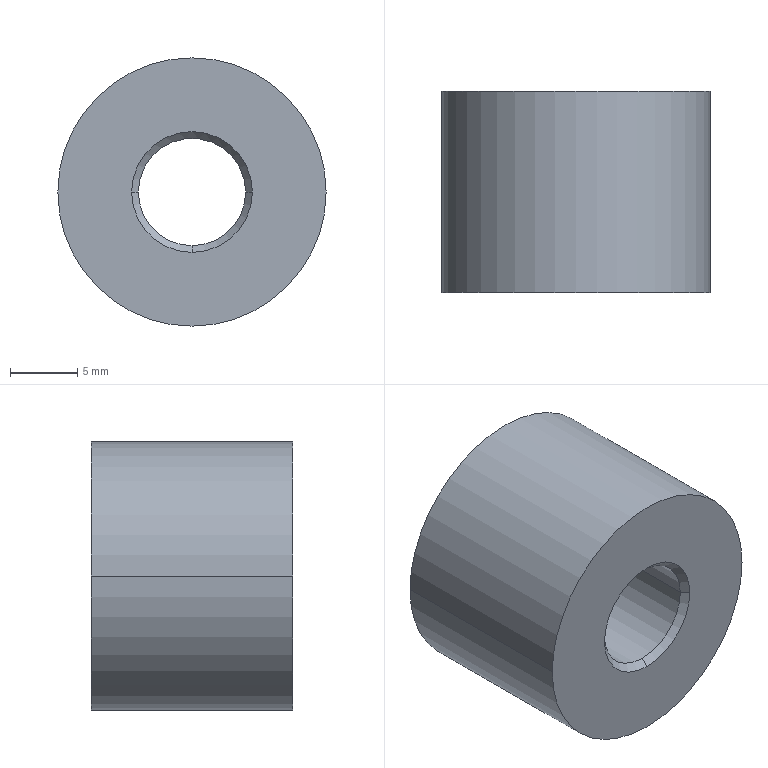Part | SolidWorks | features BaseBody 1 | 1 solid | 12 faces | box 20 x 15 x 20 mm | volume 3952 mm3 | cone 6 | cylinder 4 | plane 2 | commonest cylinder face diameters 8 x2 20 x2
STEP:
#1=CARTESIAN_POINT('',(-4.5,0.,0.));
#2=VERTEX_POINT('',#1);
#3=CARTESIAN_POINT('',(0.,0.,-4.5));
#4=VERTEX_POINT('',#3);
#5=CARTESIAN_POINT('',(0.,0.,0.));
#6=DIRECTION('',(0.,-1.,0.));
#7=DIRECTION('',(0.,0.,-1.));
#8=AXIS2_PLACEMENT_3D('',#5,#6,#7);
#9=CIRCLE('',#8,4.5);
#10=EDGE_CURVE('',#2,#4,#9,.T.);
#11=ORIENTED_EDGE('',*,*,#10,.F.);
#12=CARTESIAN_POINT('',(4.5,0.,0.));
#13=VERTEX_POINT('',#12);
#14=CARTESIAN_POINT('',(0.,0.,0.));
#15=DIRECTION('',(0.,-1.,0.));
#16=DIRECTION('',(0.,0.,1.));
#17=AXIS2_PLACEMENT_3D('',#14,#15,#16);
#18=CIRCLE('',#17,4.5);
#19=EDGE_CURVE('',#13,#2,#18,.T.);
#20=ORIENTED_EDGE('',*,*,#19,.F.);
#21=CARTESIAN_POINT('',(0.,0.,0.));
#22=DIRECTION('',(0.,-1.,0.));
#23=DIRECTION('',(0.,0.,-1.));
#24=AXIS2_PLACEMENT_3D('',#21,#22,#23);
#25=CIRCLE('',#24,4.5);
#26=EDGE_CURVE('',#4,#13,#25,.T.);
#27=ORIENTED_EDGE('',*,*,#26,.F.);
#28=EDGE_LOOP('',(#11,#20,#27));
#29=FACE_BOUND('',#28,.T.);
#30=CARTESIAN_POINT('',(10.,0.,0.));
#31=VERTEX_POINT('',#30);
#32=CARTESIAN_POINT('',(-10.,0.,0.));
#33=VERTEX_POINT('',#32);
#34=CARTESIAN_POINT('',(0.,0.,0.));
#35=DIRECTION('',(0.,1.,0.));
#36=DIRECTION('',(1.,0.,0.));
#37=AXIS2_PLACEMENT_3D('',#34,#35,#36);
#38=CIRCLE('',#37,10.);
#39=EDGE_CURVE('',#31,#33,#38,.T.);
#40=ORIENTED_EDGE('',*,*,#39,.F.);
#41=CARTESIAN_POINT('',(0.,0.,0.));
#42=DIRECTION('',(0.,1.,0.));
#43=DIRECTION('',(-1.,0.,0.));
#44=AXIS2_PLACEMENT_3D('',#41,#42,#43);
#45=CIRCLE('',#44,10.);
#46=EDGE_CURVE('',#33,#31,#45,.T.);
#47=ORIENTED_EDGE('',*,*,#46,.F.);
#48=EDGE_LOOP('',(#40,#47));
#49=FACE_OUTER_BOUND('',#48,.T.);
#50=CARTESIAN_POINT('',(0.,0.,0.));
#51=DIRECTION('',(0.,1.,0.));
#52=DIRECTION('',(1.,0.,0.));
#53=AXIS2_PLACEMENT_3D('',#50,#51,#52);
#54=PLANE('',#53);
#55=ADVANCED_FACE('',(#29,#49),#54,.F.);
#56=CARTESIAN_POINT('',(10.,15.,0.));
#57=VERTEX_POINT('',#56);
#58=CARTESIAN_POINT('',(-10.,15.,0.));
#59=VERTEX_POINT('',#58);
#60=CARTESIAN_POINT('',(0.,15.,0.));
#61=DIRECTION('',(0.,-1.,0.));
#62=DIRECTION('',(1.,0.,0.));
#63=AXIS2_PLACEMENT_3D('',#60,#61,#62);
#64=CIRCLE('',#63,10.);
#65=EDGE_CURVE('',#57,#59,#64,.T.);
#66=ORIENTED_EDGE('',*,*,#65,.T.);
#67=CARTESIAN_POINT('',(-10.,15.,0.));
#68=DIRECTION('',(0.,-1.,0.));
#69=VECTOR('',#68,1000.);
#70=LINE('',#67,#69);
#71=EDGE_CURVE('',#59,#33,#70,.T.);
#72=ORIENTED_EDGE('',*,*,#71,.T.);
#73=ORIENTED_EDGE('',*,*,#46,.T.);
#74=CARTESIAN_POINT('',(10.,15.,0.));
#75=DIRECTION('',(0.,-1.,0.));
#76=VECTOR('',#75,1000.);
#77=LINE('',#74,#76);
#78=EDGE_CURVE('',#57,#31,#77,.T.);
#79=ORIENTED_EDGE('',*,*,#78,.F.);
#80=EDGE_LOOP('',(#66,#72,#73,#79));
#81=FACE_OUTER_BOUND('',#80,.T.);
#82=CARTESIAN_POINT('',(0.,-0.75,0.));
#83=DIRECTION('',(0.,1.,0.));
#84=DIRECTION('',(1.,0.,0.));
#85=AXIS2_PLACEMENT_3D('',#82,#83,#84);
#86=CYLINDRICAL_SURFACE('',#85,10.);
#87=ADVANCED_FACE('',(#81),#86,.T.);
#88=ORIENTED_EDGE('',*,*,#39,.T.);
#89=ORIENTED_EDGE('',*,*,#71,.F.);
#90=CARTESIAN_POINT('',(0.,15.,0.));
#91=DIRECTION('',(0.,-1.,0.));
#92=DIRECTION('',(-1.,0.,0.));
#93=AXIS2_PLACEMENT_3D('',#90,#91,#92);
#94=CIRCLE('',#93,10.);
#95=EDGE_CURVE('',#59,#57,#94,.T.);
#96=ORIENTED_EDGE('',*,*,#95,.T.);
#97=ORIENTED_EDGE('',*,*,#78,.T.);
#98=EDGE_LOOP('',(#88,#89,#96,#97));
#99=FACE_OUTER_BOUND('',#98,.T.);
#100=CARTESIAN_POINT('',(0.,-0.75,0.));
#101=DIRECTION('',(0.,1.,0.));
#102=DIRECTION('',(1.,0.,0.));
#103=AXIS2_PLACEMENT_3D('',#100,#101,#102);
#104=CYLINDRICAL_SURFACE('',#103,10.);
#105=ADVANCED_FACE('',(#99),#104,.T.);
#106=CARTESIAN_POINT('',(4.5,15.,0.));
#107=VERTEX_POINT('',#106);
#108=CARTESIAN_POINT('',(0.,15.,-4.5));
#109=VERTEX_POINT('',#108);
#110=CARTESIAN_POINT('',(0.,15.,0.));
#111=DIRECTION('',(0.,1.,0.));
#112=DIRECTION('',(0.,0.,-1.));
#113=AXIS2_PLACEMENT_3D('',#110,#111,#112);
#114=CIRCLE('',#113,4.5);
#115=EDGE_CURVE('',#107,#109,#114,.T.);
#116=ORIENTED_EDGE('',*,*,#115,.F.);
#117=CARTESIAN_POINT('',(-4.5,15.,0.));
#118=VERTEX_POINT('',#117);
#119=CARTESIAN_POINT('',(0.,15.,0.));
#120=DIRECTION('',(0.,1.,0.));
#121=DIRECTION('',(0.,0.,1.));
#122=AXIS2_PLACEMENT_3D('',#119,#120,#121);
#123=CIRCLE('',#122,4.5);
#124=EDGE_CURVE('',#118,#107,#123,.T.);
#125=ORIENTED_EDGE('',*,*,#124,.F.);
#126=CARTESIAN_POINT('',(0.,15.,0.));
#127=DIRECTION('',(0.,1.,0.));
#128=DIRECTION('',(0.,0.,-1.));
#129=AXIS2_PLACEMENT_3D('',#126,#127,#128);
#130=CIRCLE('',#129,4.5);
#131=EDGE_CURVE('',#109,#118,#130,.T.);
#132=ORIENTED_EDGE('',*,*,#131,.F.);
#133=EDGE_LOOP('',(#116,#125,#132));
#134=FACE_BOUND('',#133,.T.);
#135=ORIENTED_EDGE('',*,*,#65,.F.);
#136=ORIENTED_EDGE('',*,*,#95,.F.);
#137=EDGE_LOOP('',(#135,#136));
#138=FACE_OUTER_BOUND('',#137,.T.);
#139=CARTESIAN_POINT('',(0.,15.,0.));
#140=DIRECTION('',(0.,1.,0.));
#141=DIRECTION('',(1.,0.,0.));
#142=AXIS2_PLACEMENT_3D('',#139,#140,#141);
#143=PLANE('',#142);
#144=ADVANCED_FACE('',(#134,#138),#143,.T.);
#145=CARTESIAN_POINT('',(-4.,14.5,-0.000000043));
#146=VERTEX_POINT('',#145);
#147=CARTESIAN_POINT('',(-4.5,15.,0.000000007));
#148=DIRECTION('',(0.7071,-0.7071,-0.000000034));
#149=VECTOR('',#148,1000.);
#150=LINE('',#147,#149);
#151=EDGE_CURVE('',#118,#146,#150,.T.);
#152=ORIENTED_EDGE('',*,*,#151,.F.);
#153=ORIENTED_EDGE('',*,*,#124,.T.);
#154=CARTESIAN_POINT('',(4.,14.5,0.));
#155=VERTEX_POINT('',#154);
#156=CARTESIAN_POINT('',(4.5,15.,-0.000000007));
#157=DIRECTION('',(-0.7071,-0.7071,0.000000003));
#158=VECTOR('',#157,1000.);
#159=LINE('',#156,#158);
#160=EDGE_CURVE('',#107,#155,#159,.T.);
#161=ORIENTED_EDGE('',*,*,#160,.T.);
#162=CARTESIAN_POINT('',(0.,14.5,0.));
#163=DIRECTION('',(0.,1.,0.));
#164=DIRECTION('',(0.,0.,1.));
#165=AXIS2_PLACEMENT_3D('',#162,#163,#164);
#166=CIRCLE('',#165,4.);
#167=EDGE_CURVE('',#146,#155,#166,.T.);
#168=ORIENTED_EDGE('',*,*,#167,.F.);
#169=EDGE_LOOP('',(#152,#153,#161,#168));
#170=FACE_OUTER_BOUND('',#169,.T.);
#171=CARTESIAN_POINT('',(0.,14.75,0.));
#172=DIRECTION('',(0.,1.,0.));
#173=DIRECTION('',(0.,0.,-1.));
#174=AXIS2_PLACEMENT_3D('',#171,#172,#173);
#175=CONICAL_SURFACE('',#174,4.25,0.7854);
#176=ADVANCED_FACE('',(#170),#175,.F.);
#177=CARTESIAN_POINT('',(4.,0.5,0.));
#178=VERTEX_POINT('',#177);
#179=CARTESIAN_POINT('',(4.,0.5,0.000000055));
#180=DIRECTION('',(0.,1.,-0.000000004));
#181=VECTOR('',#180,1000.);
#182=LINE('',#179,#181);
#183=EDGE_CURVE('',#178,#155,#182,.T.);
#184=ORIENTED_EDGE('',*,*,#183,.F.);
#185=CARTESIAN_POINT('',(-4.,0.5,-0.000000077));
#186=VERTEX_POINT('',#185);
#187=CARTESIAN_POINT('',(0.,0.5,0.));
#188=DIRECTION('',(0.,-1.,0.));
#189=DIRECTION('',(1.,0.,0.));
#190=AXIS2_PLACEMENT_3D('',#187,#188,#189);
#191=CIRCLE('',#190,4.);
#192=EDGE_CURVE('',#178,#186,#191,.T.);
#193=ORIENTED_EDGE('',*,*,#192,.T.);
#194=CARTESIAN_POINT('',(-4.,0.5,-0.000000077));
#195=DIRECTION('',(0.,1.,0.000000004));
#196=VECTOR('',#195,1000.);
#197=LINE('',#194,#196);
#198=EDGE_CURVE('',#186,#146,#197,.T.);
#199=ORIENTED_EDGE('',*,*,#198,.T.);
#200=ORIENTED_EDGE('',*,*,#167,.T.);
#201=EDGE_LOOP('',(#184,#193,#199,#200));
#202=FACE_OUTER_BOUND('',#201,.T.);
#203=CARTESIAN_POINT('',(0.,-0.75,0.));
#204=DIRECTION('',(0.,1.,0.));
#205=DIRECTION('',(1.,0.,0.));
#206=AXIS2_PLACEMENT_3D('',#203,#204,#205);
#207=CYLINDRICAL_SURFACE('',#206,4.);
#208=ADVANCED_FACE('',(#202),#207,.F.);
#209=ORIENTED_EDGE('',*,*,#198,.F.);
#210=CARTESIAN_POINT('',(0.,0.5,-4.));
#211=VERTEX_POINT('',#210);
#212=CARTESIAN_POINT('',(0.,0.5,0.));
#213=DIRECTION('',(0.,-1.,0.));
#214=DIRECTION('',(-1.,0.,-0.000000011));
#215=AXIS2_PLACEMENT_3D('',#212,#213,#214);
#216=CIRCLE('',#215,4.);
#217=EDGE_CURVE('',#186,#211,#216,.T.);
#218=ORIENTED_EDGE('',*,*,#217,.T.);
#219=CARTESIAN_POINT('',(0.,0.5,0.));
#220=DIRECTION('',(0.,-1.,0.));
#221=DIRECTION('',(-1.,0.,-0.000000011));
#222=AXIS2_PLACEMENT_3D('',#219,#220,#221);
#223=CIRCLE('',#222,4.);
#224=EDGE_CURVE('',#211,#178,#223,.T.);
#225=ORIENTED_EDGE('',*,*,#224,.T.);
#226=ORIENTED_EDGE('',*,*,#183,.T.);
#227=CARTESIAN_POINT('',(0.,14.5,-4.));
#228=VERTEX_POINT('',#227);
#229=CARTESIAN_POINT('',(0.,14.5,0.));
#230=DIRECTION('',(0.,1.,0.));
#231=DIRECTION('',(1.,0.,0.));
#232=AXIS2_PLACEMENT_3D('',#229,#230,#231);
#233=CIRCLE('',#232,4.);
#234=EDGE_CURVE('',#155,#228,#233,.T.);
#235=ORIENTED_EDGE('',*,*,#234,.T.);
#236=CARTESIAN_POINT('',(0.,14.5,0.));
#237=DIRECTION('',(0.,1.,0.));
#238=DIRECTION('',(1.,0.,0.));
#239=AXIS2_PLACEMENT_3D('',#236,#237,#238);
#240=CIRCLE('',#239,4.);
#241=EDGE_CURVE('',#228,#146,#240,.T.);
#242=ORIENTED_EDGE('',*,*,#241,.T.);
#243=EDGE_LOOP('',(#209,#218,#225,#226,#235,#242));
#244=FACE_OUTER_BOUND('',#243,.T.);
#245=CARTESIAN_POINT('',(0.,-0.75,0.));
#246=DIRECTION('',(0.,1.,0.));
#247=DIRECTION('',(1.,0.,0.));
#248=AXIS2_PLACEMENT_3D('',#245,#246,#247);
#249=CYLINDRICAL_SURFACE('',#248,4.);
#250=ADVANCED_FACE('',(#244),#249,.F.);
#251=CARTESIAN_POINT('',(0.,14.75,-4.25));
#252=DIRECTION('',(0.,0.7071,-0.7071));
#253=VECTOR('',#252,1000.);
#254=LINE('',#251,#253);
#255=EDGE_CURVE('',#228,#109,#254,.T.);
#256=ORIENTED_EDGE('',*,*,#255,.F.);
#257=ORIENTED_EDGE('',*,*,#234,.F.);
#258=ORIENTED_EDGE('',*,*,#160,.F.);
#259=ORIENTED_EDGE('',*,*,#115,.T.);
#260=EDGE_LOOP('',(#256,#257,#258,#259));
#261=FACE_OUTER_BOUND('',#260,.T.);
#262=CARTESIAN_POINT('',(0.,14.75,0.));
#263=DIRECTION('',(0.,1.,0.));
#264=DIRECTION('',(0.,0.,-1.));
#265=AXIS2_PLACEMENT_3D('',#262,#263,#264);
#266=CONICAL_SURFACE('',#265,4.25,0.7854);
#267=ADVANCED_FACE('',(#261),#266,.F.);
#268=CARTESIAN_POINT('',(0.,0.25,-4.25));
#269=DIRECTION('',(0.,-0.7071,-0.7071));
#270=VECTOR('',#269,1000.);
#271=LINE('',#268,#270);
#272=EDGE_CURVE('',#211,#4,#271,.T.);
#273=ORIENTED_EDGE('',*,*,#272,.F.);
#274=ORIENTED_EDGE('',*,*,#217,.F.);
#275=CARTESIAN_POINT('',(-4.,0.5,-0.000000077));
#276=DIRECTION('',(-0.7071,-0.7071,-0.000000009));
#277=VECTOR('',#276,1000.);
#278=LINE('',#275,#277);
#279=EDGE_CURVE('',#186,#2,#278,.T.);
#280=ORIENTED_EDGE('',*,*,#279,.T.);
#281=ORIENTED_EDGE('',*,*,#10,.T.);
#282=EDGE_LOOP('',(#273,#274,#280,#281));
#283=FACE_OUTER_BOUND('',#282,.T.);
#284=CARTESIAN_POINT('',(0.,0.25,0.));
#285=DIRECTION('',(0.,-1.,0.));
#286=DIRECTION('',(0.,0.,-1.));
#287=AXIS2_PLACEMENT_3D('',#284,#285,#286);
#288=CONICAL_SURFACE('',#287,4.25,0.7854);
#289=ADVANCED_FACE('',(#283),#288,.F.);
#290=ORIENTED_EDGE('',*,*,#279,.F.);
#291=ORIENTED_EDGE('',*,*,#192,.F.);
#292=CARTESIAN_POINT('',(4.,0.5,0.000000055));
#293=DIRECTION('',(0.7071,-0.7071,0.000000039));
#294=VECTOR('',#293,1000.);
#295=LINE('',#292,#294);
#296=EDGE_CURVE('',#178,#13,#295,.T.);
#297=ORIENTED_EDGE('',*,*,#296,.T.);
#298=ORIENTED_EDGE('',*,*,#19,.T.);
#299=EDGE_LOOP('',(#290,#291,#297,#298));
#300=FACE_OUTER_BOUND('',#299,.T.);
#301=CARTESIAN_POINT('',(0.,0.25,0.));
#302=DIRECTION('',(0.,-1.,0.));
#303=DIRECTION('',(0.,0.,-1.));
#304=AXIS2_PLACEMENT_3D('',#301,#302,#303);
#305=CONICAL_SURFACE('',#304,4.25,0.7854);
#306=ADVANCED_FACE('',(#300),#305,.F.);
#307=ORIENTED_EDGE('',*,*,#224,.F.);
#308=ORIENTED_EDGE('',*,*,#272,.T.);
#309=ORIENTED_EDGE('',*,*,#26,.T.);
#310=ORIENTED_EDGE('',*,*,#296,.F.);
#311=EDGE_LOOP('',(#307,#308,#309,#310));
#312=FACE_OUTER_BOUND('',#311,.T.);
#313=CARTESIAN_POINT('',(0.,0.25,0.));
#314=DIRECTION('',(0.,-1.,0.));
#315=DIRECTION('',(0.,0.,-1.));
#316=AXIS2_PLACEMENT_3D('',#313,#314,#315);
#317=CONICAL_SURFACE('',#316,4.25,0.7854);
#318=ADVANCED_FACE('',(#312),#317,.F.);
#319=ORIENTED_EDGE('',*,*,#241,.F.);
#320=ORIENTED_EDGE('',*,*,#255,.T.);
#321=ORIENTED_EDGE('',*,*,#131,.T.);
#322=ORIENTED_EDGE('',*,*,#151,.T.);
#323=EDGE_LOOP('',(#319,#320,#321,#322));
#324=FACE_OUTER_BOUND('',#323,.T.);
#325=CARTESIAN_POINT('',(0.,14.75,0.));
#326=DIRECTION('',(0.,1.,0.));
#327=DIRECTION('',(0.,0.,-1.));
#328=AXIS2_PLACEMENT_3D('',#325,#326,#327);
#329=CONICAL_SURFACE('',#328,4.25,0.7854);
#330=ADVANCED_FACE('',(#324),#329,.F.);
#331=CLOSED_SHELL('',(#55,#87,#105,#144,#176,#208,#250,#267,#289,#306,#318,#330));
#332=MANIFOLD_SOLID_BREP('',#331);
#333=CARTESIAN_POINT('',(0.,0.,0.));
#334=DIRECTION('',(0.,0.,1.));
#335=DIRECTION('',(1.,0.,0.));
#336=AXIS2_PLACEMENT_3D('',#333,#334,#335);
#337=(LENGTH_UNIT()NAMED_UNIT(*)SI_UNIT(.MILLI.,.METRE.));
#338=UNCERTAINTY_MEASURE_WITH_UNIT(LENGTH_MEASURE(0.00001),#337,'','');
#339=(NAMED_UNIT(*)PLANE_ANGLE_UNIT()SI_UNIT($,.RADIAN.));
#340=(NAMED_UNIT(*)SI_UNIT($,.STERADIAN.)SOLID_ANGLE_UNIT());
#341=(GEOMETRIC_REPRESENTATION_CONTEXT(3)GLOBAL_UNCERTAINTY_ASSIGNED_CONTEXT((#338))GLOBAL_UNIT_ASSIGNED_CONTEXT((#337,#339,#340))REPRESENTATION_CONTEXT('',''));
#342=ADVANCED_BREP_SHAPE_REPRESENTATION('',(#332,#336),#341);